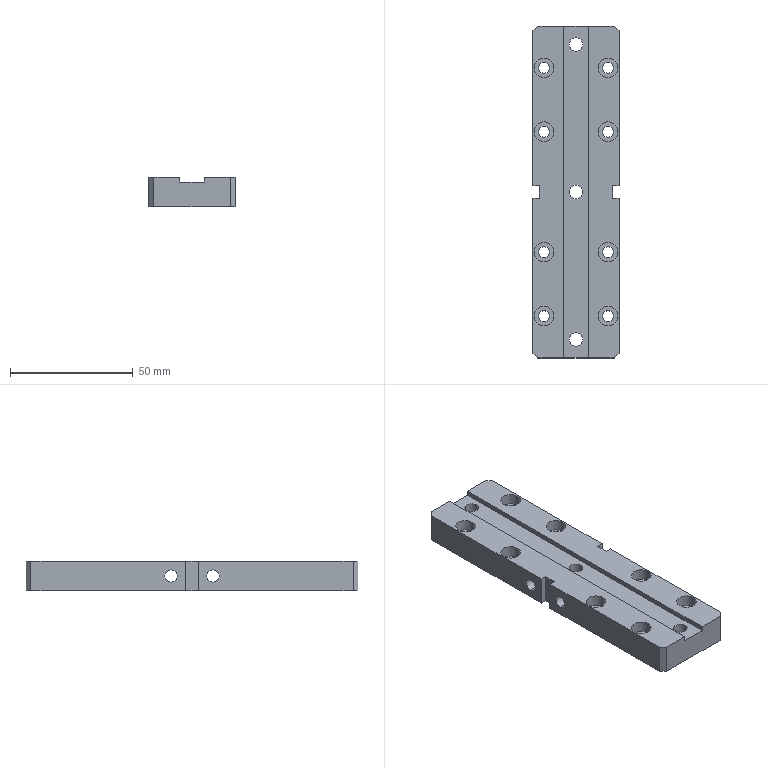Part | SolidWorks | features BaseBody 1 | 1 solid | 81 faces | box 35 x 135 x 12 mm | volume 47871 mm3 | cylinder 48 | plane 33 | commonest cylinder face diameters 4.5 x16 8 x16 5.5 x6 10 x6 5 x4